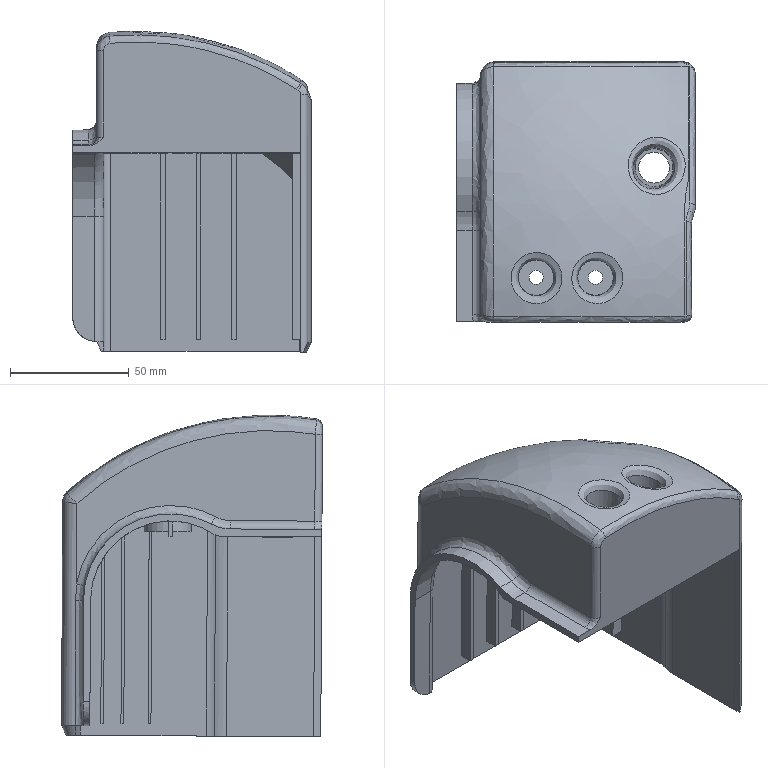Part | STEP file | EDN CAP NQ7A | 1 solid | 148 faces | box 100.427 x 109.896 x 135.338 mm | volume 139649 mm3 | plane 79 | spline 32 | cylinder 31 | cone 4 | torus 2 | commonest cylinder face diameters 20 x8 6 x5 8 x3 13 x3 15 x2 4 x1